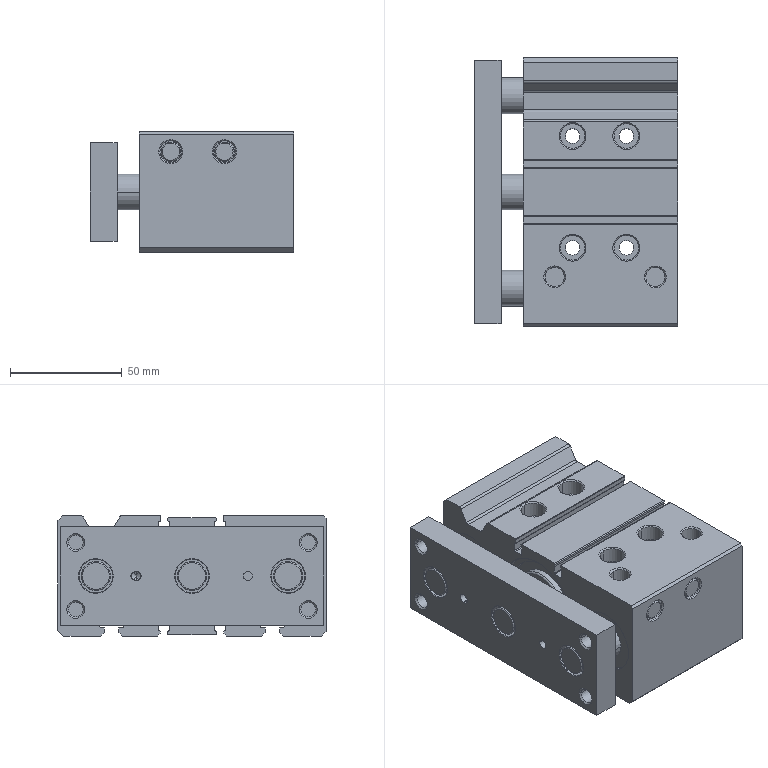Part | SolidWorks | 2 solids | 382 faces | box 91 x 120 x 54 mm | volume 409474 mm3 | cylinder 167 | plane 117 | cone 88 | torus 10 | commonest cylinder face diameters 0.8 x28 6.647 x24 4 x21 0.4 x12 16 x12 6.5 x8